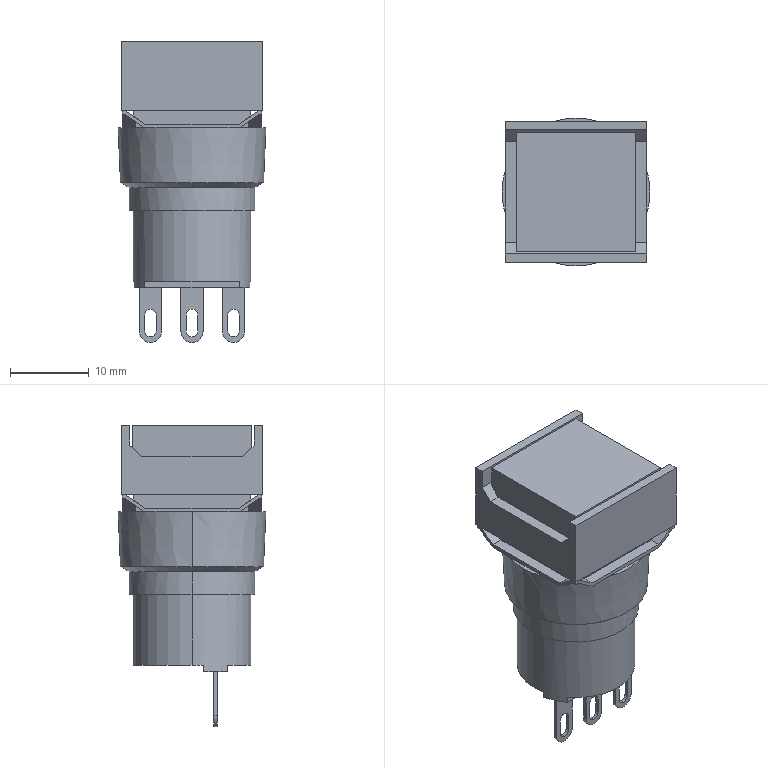Part | STEP file | Button | 1 solid | 111 faces | box 18.8 x 18.8 x 38.3 mm | volume 7439 mm3 | plane 91 | cylinder 16 | cone 4 | commonest cylinder face diameters 1.5 x9 2.8 x3 15 x2 16 x2